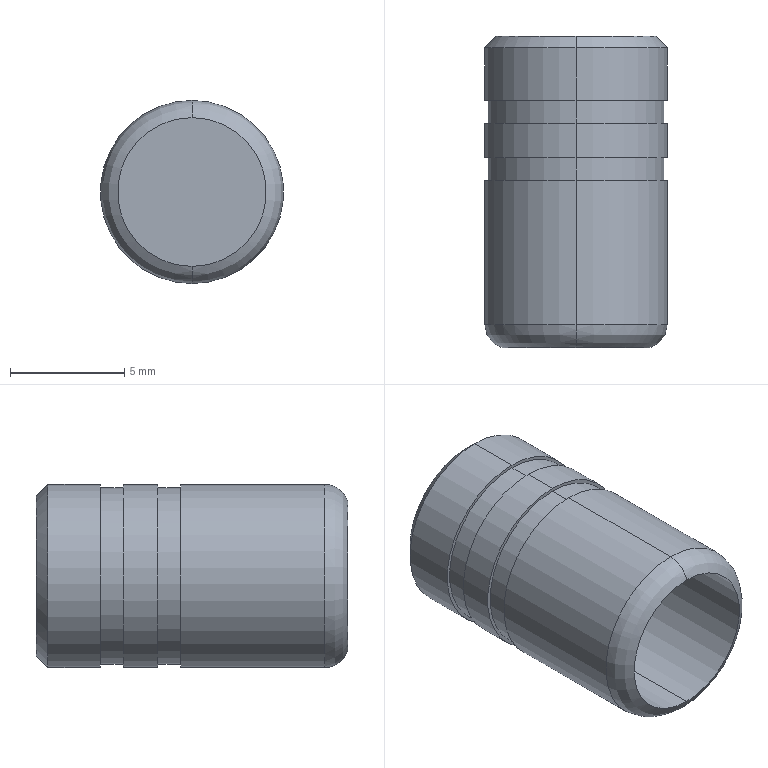Part | SolidWorks | features Revolution 1 | 1 solid | 25 faces | box 8 x 13.6 x 8 mm | volume 252.417 mm3 | cylinder 12 | plane 7 | cone 4 | torus 2 | commonest cylinder face diameters 8 x6 7.7 x4 6.5 x2
STEP:
#1=CARTESIAN_POINT('',(0.,7.3,-4.));
#2=VERTEX_POINT('',#1);
#3=CARTESIAN_POINT('',(0.,7.3,4.));
#4=VERTEX_POINT('',#3);
#5=CARTESIAN_POINT('',(0.,7.3,0.));
#6=DIRECTION('',(0.,-1.,0.));
#7=DIRECTION('',(0.,0.,-1.));
#8=AXIS2_PLACEMENT_3D('',#5,#6,#7);
#9=CIRCLE('',#8,4.);
#10=EDGE_CURVE('',#2,#4,#9,.T.);
#11=ORIENTED_EDGE('',*,*,#10,.T.);
#12=CARTESIAN_POINT('',(0.,1.,4.));
#13=VERTEX_POINT('',#12);
#14=CARTESIAN_POINT('',(0.,0.,4.));
#15=DIRECTION('',(0.,-1.,0.));
#16=VECTOR('',#15,1000.);
#17=LINE('',#14,#16);
#18=EDGE_CURVE('',#4,#13,#17,.T.);
#19=ORIENTED_EDGE('',*,*,#18,.T.);
#20=CARTESIAN_POINT('',(0.,1.,-4.));
#21=VERTEX_POINT('',#20);
#22=CARTESIAN_POINT('',(0.,1.,0.));
#23=DIRECTION('',(0.,-1.,0.));
#24=DIRECTION('',(0.,0.,-1.));
#25=AXIS2_PLACEMENT_3D('',#22,#23,#24);
#26=CIRCLE('',#25,4.);
#27=EDGE_CURVE('',#21,#13,#26,.T.);
#28=ORIENTED_EDGE('',*,*,#27,.F.);
#29=CARTESIAN_POINT('',(0.,0.,-4.));
#30=DIRECTION('',(0.,-1.,0.));
#31=VECTOR('',#30,1000.);
#32=LINE('',#29,#31);
#33=EDGE_CURVE('',#2,#21,#32,.T.);
#34=ORIENTED_EDGE('',*,*,#33,.F.);
#35=EDGE_LOOP('',(#11,#19,#28,#34));
#36=FACE_OUTER_BOUND('',#35,.T.);
#37=CARTESIAN_POINT('',(0.,0.,0.));
#38=DIRECTION('',(0.,-1.,0.));
#39=DIRECTION('',(0.,0.,-1.));
#40=AXIS2_PLACEMENT_3D('',#37,#38,#39);
#41=CYLINDRICAL_SURFACE('',#40,4.);
#42=ADVANCED_FACE('',(#36),#41,.T.);
#43=CARTESIAN_POINT('',(0.,8.3,-3.85));
#44=VERTEX_POINT('',#43);
#45=CARTESIAN_POINT('',(0.,8.3,3.85));
#46=VERTEX_POINT('',#45);
#47=CARTESIAN_POINT('',(0.,8.3,0.));
#48=DIRECTION('',(0.,-1.,0.));
#49=DIRECTION('',(0.,0.,-1.));
#50=AXIS2_PLACEMENT_3D('',#47,#48,#49);
#51=CIRCLE('',#50,3.85);
#52=EDGE_CURVE('',#44,#46,#51,.T.);
#53=ORIENTED_EDGE('',*,*,#52,.T.);
#54=CARTESIAN_POINT('',(0.,7.3,3.85));
#55=VERTEX_POINT('',#54);
#56=CARTESIAN_POINT('',(0.,0.,3.85));
#57=DIRECTION('',(0.,-1.,0.));
#58=VECTOR('',#57,1000.);
#59=LINE('',#56,#58);
#60=EDGE_CURVE('',#46,#55,#59,.T.);
#61=ORIENTED_EDGE('',*,*,#60,.T.);
#62=CARTESIAN_POINT('',(0.,7.3,-3.85));
#63=VERTEX_POINT('',#62);
#64=CARTESIAN_POINT('',(0.,7.3,0.));
#65=DIRECTION('',(0.,-1.,0.));
#66=DIRECTION('',(0.,0.,-1.));
#67=AXIS2_PLACEMENT_3D('',#64,#65,#66);
#68=CIRCLE('',#67,3.85);
#69=EDGE_CURVE('',#63,#55,#68,.T.);
#70=ORIENTED_EDGE('',*,*,#69,.F.);
#71=CARTESIAN_POINT('',(0.,0.,-3.85));
#72=DIRECTION('',(0.,-1.,0.));
#73=VECTOR('',#72,1000.);
#74=LINE('',#71,#73);
#75=EDGE_CURVE('',#44,#63,#74,.T.);
#76=ORIENTED_EDGE('',*,*,#75,.F.);
#77=EDGE_LOOP('',(#53,#61,#70,#76));
#78=FACE_OUTER_BOUND('',#77,.T.);
#79=CARTESIAN_POINT('',(0.,0.,0.));
#80=DIRECTION('',(0.,-1.,0.));
#81=DIRECTION('',(0.,0.,-1.));
#82=AXIS2_PLACEMENT_3D('',#79,#80,#81);
#83=CYLINDRICAL_SURFACE('',#82,3.85);
#84=ADVANCED_FACE('',(#78),#83,.T.);
#85=CARTESIAN_POINT('',(0.,9.8,-4.));
#86=VERTEX_POINT('',#85);
#87=CARTESIAN_POINT('',(0.,9.8,4.));
#88=VERTEX_POINT('',#87);
#89=CARTESIAN_POINT('',(0.,9.8,0.));
#90=DIRECTION('',(0.,-1.,0.));
#91=DIRECTION('',(0.,0.,-1.));
#92=AXIS2_PLACEMENT_3D('',#89,#90,#91);
#93=CIRCLE('',#92,4.);
#94=EDGE_CURVE('',#86,#88,#93,.T.);
#95=ORIENTED_EDGE('',*,*,#94,.T.);
#96=CARTESIAN_POINT('',(0.,8.3,4.));
#97=VERTEX_POINT('',#96);
#98=CARTESIAN_POINT('',(0.,0.,4.));
#99=DIRECTION('',(0.,-1.,0.));
#100=VECTOR('',#99,1000.);
#101=LINE('',#98,#100);
#102=EDGE_CURVE('',#88,#97,#101,.T.);
#103=ORIENTED_EDGE('',*,*,#102,.T.);
#104=CARTESIAN_POINT('',(0.,8.3,-4.));
#105=VERTEX_POINT('',#104);
#106=CARTESIAN_POINT('',(0.,8.3,0.));
#107=DIRECTION('',(0.,-1.,0.));
#108=DIRECTION('',(0.,0.,-1.));
#109=AXIS2_PLACEMENT_3D('',#106,#107,#108);
#110=CIRCLE('',#109,4.);
#111=EDGE_CURVE('',#105,#97,#110,.T.);
#112=ORIENTED_EDGE('',*,*,#111,.F.);
#113=CARTESIAN_POINT('',(0.,0.,-4.));
#114=DIRECTION('',(0.,-1.,0.));
#115=VECTOR('',#114,1000.);
#116=LINE('',#113,#115);
#117=EDGE_CURVE('',#86,#105,#116,.T.);
#118=ORIENTED_EDGE('',*,*,#117,.F.);
#119=EDGE_LOOP('',(#95,#103,#112,#118));
#120=FACE_OUTER_BOUND('',#119,.T.);
#121=CARTESIAN_POINT('',(0.,0.,0.));
#122=DIRECTION('',(0.,-1.,0.));
#123=DIRECTION('',(0.,0.,-1.));
#124=AXIS2_PLACEMENT_3D('',#121,#122,#123);
#125=CYLINDRICAL_SURFACE('',#124,4.);
#126=ADVANCED_FACE('',(#120),#125,.T.);
#127=CARTESIAN_POINT('',(0.,10.8,-3.85));
#128=VERTEX_POINT('',#127);
#129=CARTESIAN_POINT('',(0.,10.8,3.85));
#130=VERTEX_POINT('',#129);
#131=CARTESIAN_POINT('',(0.,10.8,0.));
#132=DIRECTION('',(0.,-1.,0.));
#133=DIRECTION('',(0.,0.,-1.));
#134=AXIS2_PLACEMENT_3D('',#131,#132,#133);
#135=CIRCLE('',#134,3.85);
#136=EDGE_CURVE('',#128,#130,#135,.T.);
#137=ORIENTED_EDGE('',*,*,#136,.T.);
#138=CARTESIAN_POINT('',(0.,9.8,3.85));
#139=VERTEX_POINT('',#138);
#140=CARTESIAN_POINT('',(0.,0.,3.85));
#141=DIRECTION('',(0.,-1.,0.));
#142=VECTOR('',#141,1000.);
#143=LINE('',#140,#142);
#144=EDGE_CURVE('',#130,#139,#143,.T.);
#145=ORIENTED_EDGE('',*,*,#144,.T.);
#146=CARTESIAN_POINT('',(0.,9.8,-3.85));
#147=VERTEX_POINT('',#146);
#148=CARTESIAN_POINT('',(0.,9.8,0.));
#149=DIRECTION('',(0.,-1.,0.));
#150=DIRECTION('',(0.,0.,-1.));
#151=AXIS2_PLACEMENT_3D('',#148,#149,#150);
#152=CIRCLE('',#151,3.85);
#153=EDGE_CURVE('',#147,#139,#152,.T.);
#154=ORIENTED_EDGE('',*,*,#153,.F.);
#155=CARTESIAN_POINT('',(0.,0.,-3.85));
#156=DIRECTION('',(0.,-1.,0.));
#157=VECTOR('',#156,1000.);
#158=LINE('',#155,#157);
#159=EDGE_CURVE('',#128,#147,#158,.T.);
#160=ORIENTED_EDGE('',*,*,#159,.F.);
#161=EDGE_LOOP('',(#137,#145,#154,#160));
#162=FACE_OUTER_BOUND('',#161,.T.);
#163=CARTESIAN_POINT('',(0.,0.,0.));
#164=DIRECTION('',(0.,-1.,0.));
#165=DIRECTION('',(0.,0.,-1.));
#166=AXIS2_PLACEMENT_3D('',#163,#164,#165);
#167=CYLINDRICAL_SURFACE('',#166,3.85);
#168=ADVANCED_FACE('',(#162),#167,.T.);
#169=CARTESIAN_POINT('',(0.,13.1,-4.));
#170=VERTEX_POINT('',#169);
#171=CARTESIAN_POINT('',(0.,13.1,4.));
#172=VERTEX_POINT('',#171);
#173=CARTESIAN_POINT('',(0.,13.1,0.));
#174=DIRECTION('',(0.,-1.,0.));
#175=DIRECTION('',(0.,0.,-1.));
#176=AXIS2_PLACEMENT_3D('',#173,#174,#175);
#177=CIRCLE('',#176,4.);
#178=EDGE_CURVE('',#170,#172,#177,.T.);
#179=ORIENTED_EDGE('',*,*,#178,.T.);
#180=CARTESIAN_POINT('',(0.,10.8,4.));
#181=VERTEX_POINT('',#180);
#182=CARTESIAN_POINT('',(0.,0.,4.));
#183=DIRECTION('',(0.,-1.,0.));
#184=VECTOR('',#183,1000.);
#185=LINE('',#182,#184);
#186=EDGE_CURVE('',#172,#181,#185,.T.);
#187=ORIENTED_EDGE('',*,*,#186,.T.);
#188=CARTESIAN_POINT('',(0.,10.8,-4.));
#189=VERTEX_POINT('',#188);
#190=CARTESIAN_POINT('',(0.,10.8,0.));
#191=DIRECTION('',(0.,-1.,0.));
#192=DIRECTION('',(0.,0.,-1.));
#193=AXIS2_PLACEMENT_3D('',#190,#191,#192);
#194=CIRCLE('',#193,4.);
#195=EDGE_CURVE('',#189,#181,#194,.T.);
#196=ORIENTED_EDGE('',*,*,#195,.F.);
#197=CARTESIAN_POINT('',(0.,0.,-4.));
#198=DIRECTION('',(0.,-1.,0.));
#199=VECTOR('',#198,1000.);
#200=LINE('',#197,#199);
#201=EDGE_CURVE('',#170,#189,#200,.T.);
#202=ORIENTED_EDGE('',*,*,#201,.F.);
#203=EDGE_LOOP('',(#179,#187,#196,#202));
#204=FACE_OUTER_BOUND('',#203,.T.);
#205=CARTESIAN_POINT('',(0.,0.,0.));
#206=DIRECTION('',(0.,-1.,0.));
#207=DIRECTION('',(0.,0.,-1.));
#208=AXIS2_PLACEMENT_3D('',#205,#206,#207);
#209=CYLINDRICAL_SURFACE('',#208,4.);
#210=ADVANCED_FACE('',(#204),#209,.T.);
#211=CARTESIAN_POINT('',(0.,13.6,-3.5));
#212=VERTEX_POINT('',#211);
#213=CARTESIAN_POINT('',(0.,13.6,3.5));
#214=VERTEX_POINT('',#213);
#215=CARTESIAN_POINT('',(0.,13.6,0.));
#216=DIRECTION('',(0.,-1.,0.));
#217=DIRECTION('',(0.,0.,-1.));
#218=AXIS2_PLACEMENT_3D('',#215,#216,#217);
#219=CIRCLE('',#218,3.5);
#220=EDGE_CURVE('',#212,#214,#219,.T.);
#221=ORIENTED_EDGE('',*,*,#220,.T.);
#222=CARTESIAN_POINT('',(0.,13.6,3.5));
#223=DIRECTION('',(0.,-0.7071,0.7071));
#224=VECTOR('',#223,1000.);
#225=LINE('',#222,#224);
#226=EDGE_CURVE('',#214,#172,#225,.T.);
#227=ORIENTED_EDGE('',*,*,#226,.T.);
#228=ORIENTED_EDGE('',*,*,#178,.F.);
#229=CARTESIAN_POINT('',(0.,13.6,-3.5));
#230=DIRECTION('',(0.,-0.7071,-0.7071));
#231=VECTOR('',#230,1000.);
#232=LINE('',#229,#231);
#233=EDGE_CURVE('',#212,#170,#232,.T.);
#234=ORIENTED_EDGE('',*,*,#233,.F.);
#235=EDGE_LOOP('',(#221,#227,#228,#234));
#236=FACE_OUTER_BOUND('',#235,.T.);
#237=CARTESIAN_POINT('',(0.,13.6,0.));
#238=DIRECTION('',(0.,-1.,0.));
#239=DIRECTION('',(0.,0.,-1.));
#240=AXIS2_PLACEMENT_3D('',#237,#238,#239);
#241=CONICAL_SURFACE('',#240,3.5,0.7854);
#242=ADVANCED_FACE('',(#236),#241,.T.);
#243=CARTESIAN_POINT('',(0.,13.1,0.5));
#244=VERTEX_POINT('',#243);
#245=CARTESIAN_POINT('',(0.,13.1,-0.5));
#246=VERTEX_POINT('',#245);
#247=CARTESIAN_POINT('',(0.,13.1,0.));
#248=DIRECTION('',(0.,-1.,0.));
#249=DIRECTION('',(0.,0.,-1.));
#250=AXIS2_PLACEMENT_3D('',#247,#248,#249);
#251=CIRCLE('',#250,0.5);
#252=EDGE_CURVE('',#244,#246,#251,.T.);
#253=ORIENTED_EDGE('',*,*,#252,.T.);
#254=CARTESIAN_POINT('',(0.,13.6,-1.25));
#255=VERTEX_POINT('',#254);
#256=CARTESIAN_POINT('',(0.,13.1,-0.5));
#257=DIRECTION('',(0.,0.5547,-0.8321));
#258=VECTOR('',#257,1000.);
#259=LINE('',#256,#258);
#260=EDGE_CURVE('',#246,#255,#259,.T.);
#261=ORIENTED_EDGE('',*,*,#260,.T.);
#262=CARTESIAN_POINT('',(0.,13.6,1.25));
#263=VERTEX_POINT('',#262);
#264=CARTESIAN_POINT('',(0.,13.6,0.));
#265=DIRECTION('',(0.,-1.,0.));
#266=DIRECTION('',(0.,0.,-1.));
#267=AXIS2_PLACEMENT_3D('',#264,#265,#266);
#268=CIRCLE('',#267,1.25);
#269=EDGE_CURVE('',#263,#255,#268,.T.);
#270=ORIENTED_EDGE('',*,*,#269,.F.);
#271=CARTESIAN_POINT('',(0.,13.1,0.5));
#272=DIRECTION('',(0.,0.5547,0.8321));
#273=VECTOR('',#272,1000.);
#274=LINE('',#271,#273);
#275=EDGE_CURVE('',#244,#263,#274,.T.);
#276=ORIENTED_EDGE('',*,*,#275,.F.);
#277=EDGE_LOOP('',(#253,#261,#270,#276));
#278=FACE_OUTER_BOUND('',#277,.T.);
#279=CARTESIAN_POINT('',(0.,13.1,0.));
#280=DIRECTION('',(0.,1.,0.));
#281=DIRECTION('',(0.,0.,1.));
#282=AXIS2_PLACEMENT_3D('',#279,#280,#281);
#283=CONICAL_SURFACE('',#282,0.5,0.9828);
#284=ADVANCED_FACE('',(#278),#283,.F.);
#285=CARTESIAN_POINT('',(0.,12.5,3.25));
#286=VERTEX_POINT('',#285);
#287=CARTESIAN_POINT('',(0.,12.5,-3.25));
#288=VERTEX_POINT('',#287);
#289=CARTESIAN_POINT('',(0.,12.5,0.));
#290=DIRECTION('',(0.,-1.,0.));
#291=DIRECTION('',(0.,0.,-1.));
#292=AXIS2_PLACEMENT_3D('',#289,#290,#291);
#293=CIRCLE('',#292,3.25);
#294=EDGE_CURVE('',#286,#288,#293,.T.);
#295=ORIENTED_EDGE('',*,*,#294,.F.);
#296=CARTESIAN_POINT('',(0.,0.,3.25));
#297=VERTEX_POINT('',#296);
#298=CARTESIAN_POINT('',(0.,0.,3.25));
#299=DIRECTION('',(0.,-1.,0.));
#300=VECTOR('',#299,1000.);
#301=LINE('',#298,#300);
#302=EDGE_CURVE('',#286,#297,#301,.T.);
#303=ORIENTED_EDGE('',*,*,#302,.T.);
#304=CARTESIAN_POINT('',(0.,0.,-3.25));
#305=VERTEX_POINT('',#304);
#306=CARTESIAN_POINT('',(0.,0.,0.));
#307=DIRECTION('',(0.,-1.,0.));
#308=DIRECTION('',(0.,0.,-1.));
#309=AXIS2_PLACEMENT_3D('',#306,#307,#308);
#310=CIRCLE('',#309,3.25);
#311=EDGE_CURVE('',#297,#305,#310,.T.);
#312=ORIENTED_EDGE('',*,*,#311,.T.);
#313=CARTESIAN_POINT('',(0.,0.,-3.25));
#314=DIRECTION('',(0.,-1.,0.));
#315=VECTOR('',#314,1000.);
#316=LINE('',#313,#315);
#317=EDGE_CURVE('',#288,#305,#316,.T.);
#318=ORIENTED_EDGE('',*,*,#317,.F.);
#319=EDGE_LOOP('',(#295,#303,#312,#318));
#320=FACE_OUTER_BOUND('',#319,.T.);
#321=CARTESIAN_POINT('',(0.,0.,0.));
#322=DIRECTION('',(0.,-1.,0.));
#323=DIRECTION('',(0.,0.,-1.));
#324=AXIS2_PLACEMENT_3D('',#321,#322,#323);
#325=CYLINDRICAL_SURFACE('',#324,3.25);
#326=ADVANCED_FACE('',(#320),#325,.F.);
#327=ORIENTED_EDGE('',*,*,#27,.T.);
#328=CARTESIAN_POINT('',(0.,1.,2.958));
#329=DIRECTION('',(1.,0.,0.));
#330=DIRECTION('',(0.,0.,-1.));
#331=AXIS2_PLACEMENT_3D('',#328,#329,#330);
#332=CIRCLE('',#331,1.042);
#333=EDGE_CURVE('',#13,#297,#332,.T.);
#334=ORIENTED_EDGE('',*,*,#333,.T.);
#335=CARTESIAN_POINT('',(0.,0.,0.));
#336=DIRECTION('',(0.,-1.,0.));
#337=DIRECTION('',(0.,0.,-1.));
#338=AXIS2_PLACEMENT_3D('',#335,#336,#337);
#339=CIRCLE('',#338,3.25);
#340=EDGE_CURVE('',#305,#297,#339,.T.);
#341=ORIENTED_EDGE('',*,*,#340,.F.);
#342=CARTESIAN_POINT('',(0.,1.,-2.958));
#343=DIRECTION('',(-1.,0.,0.));
#344=DIRECTION('',(0.,0.,1.));
#345=AXIS2_PLACEMENT_3D('',#342,#343,#344);
#346=CIRCLE('',#345,1.042);
#347=EDGE_CURVE('',#21,#305,#346,.T.);
#348=ORIENTED_EDGE('',*,*,#347,.F.);
#349=EDGE_LOOP('',(#327,#334,#341,#348));
#350=FACE_OUTER_BOUND('',#349,.T.);
#351=CARTESIAN_POINT('',(0.,1.,0.));
#352=DIRECTION('',(0.,-1.,0.));
#353=DIRECTION('',(0.,0.,-1.));
#354=AXIS2_PLACEMENT_3D('',#351,#352,#353);
#355=TOROIDAL_SURFACE('',#354,2.958,1.042);
#356=ADVANCED_FACE('',(#350),#355,.T.);
#357=ORIENTED_EDGE('',*,*,#333,.F.);
#358=CARTESIAN_POINT('',(0.,1.,0.));
#359=DIRECTION('',(0.,-1.,0.));
#360=DIRECTION('',(0.,0.,-1.));
#361=AXIS2_PLACEMENT_3D('',#358,#359,#360);
#362=CIRCLE('',#361,4.);
#363=EDGE_CURVE('',#13,#21,#362,.T.);
#364=ORIENTED_EDGE('',*,*,#363,.T.);
#365=ORIENTED_EDGE('',*,*,#347,.T.);
#366=ORIENTED_EDGE('',*,*,#311,.F.);
#367=EDGE_LOOP('',(#357,#364,#365,#366));
#368=FACE_OUTER_BOUND('',#367,.T.);
#369=CARTESIAN_POINT('',(0.,1.,0.));
#370=DIRECTION('',(0.,-1.,0.));
#371=DIRECTION('',(0.,0.,-1.));
#372=AXIS2_PLACEMENT_3D('',#369,#370,#371);
#373=TOROIDAL_SURFACE('',#372,2.958,1.042);
#374=ADVANCED_FACE('',(#368),#373,.T.);
#375=ORIENTED_EDGE('',*,*,#302,.F.);
#376=CARTESIAN_POINT('',(0.,12.5,0.));
#377=DIRECTION('',(0.,-1.,0.));
#378=DIRECTION('',(0.,0.,-1.));
#379=AXIS2_PLACEMENT_3D('',#376,#377,#378);
#380=CIRCLE('',#379,3.25);
#381=EDGE_CURVE('',#288,#286,#380,.T.);
#382=ORIENTED_EDGE('',*,*,#381,.F.);
#383=ORIENTED_EDGE('',*,*,#317,.T.);
#384=ORIENTED_EDGE('',*,*,#340,.T.);
#385=EDGE_LOOP('',(#375,#382,#383,#384));
#386=FACE_OUTER_BOUND('',#385,.T.);
#387=CARTESIAN_POINT('',(0.,0.,0.));
#388=DIRECTION('',(0.,-1.,0.));
#389=DIRECTION('',(0.,0.,-1.));
#390=AXIS2_PLACEMENT_3D('',#387,#388,#389);
#391=CYLINDRICAL_SURFACE('',#390,3.25);
#392=ADVANCED_FACE('',(#386),#391,.F.);
#393=ORIENTED_EDGE('',*,*,#381,.T.);
#394=ORIENTED_EDGE('',*,*,#294,.T.);
#395=EDGE_LOOP('',(#393,#394));
#396=FACE_OUTER_BOUND('',#395,.T.);
#397=CARTESIAN_POINT('',(-3.25,12.5,0.));
#398=DIRECTION('',(0.,1.,0.));
#399=DIRECTION('',(0.,0.,1.));
#400=AXIS2_PLACEMENT_3D('',#397,#398,#399);
#401=PLANE('',#400);
#402=ADVANCED_FACE('',(#396),#401,.F.);
#403=ORIENTED_EDGE('',*,*,#252,.F.);
#404=CARTESIAN_POINT('',(0.,13.1,0.));
#405=DIRECTION('',(0.,-1.,0.));
#406=DIRECTION('',(0.,0.,-1.));
#407=AXIS2_PLACEMENT_3D('',#404,#405,#406);
#408=CIRCLE('',#407,0.5);
#409=EDGE_CURVE('',#246,#244,#408,.T.);
#410=ORIENTED_EDGE('',*,*,#409,.F.);
#411=EDGE_LOOP('',(#403,#410));
#412=FACE_OUTER_BOUND('',#411,.T.);
#413=CARTESIAN_POINT('',(-0.5,13.1,0.));
#414=DIRECTION('',(0.,-1.,0.));
#415=DIRECTION('',(0.,0.,-1.));
#416=AXIS2_PLACEMENT_3D('',#413,#414,#415);
#417=PLANE('',#416);
#418=ADVANCED_FACE('',(#412),#417,.F.);
#419=ORIENTED_EDGE('',*,*,#260,.F.);
#420=ORIENTED_EDGE('',*,*,#409,.T.);
#421=ORIENTED_EDGE('',*,*,#275,.T.);
#422=CARTESIAN_POINT('',(0.,13.6,0.));
#423=DIRECTION('',(0.,-1.,0.));
#424=DIRECTION('',(0.,0.,-1.));
#425=AXIS2_PLACEMENT_3D('',#422,#423,#424);
#426=CIRCLE('',#425,1.25);
#427=EDGE_CURVE('',#255,#263,#426,.T.);
#428=ORIENTED_EDGE('',*,*,#427,.F.);
#429=EDGE_LOOP('',(#419,#420,#421,#428));
#430=FACE_OUTER_BOUND('',#429,.T.);
#431=CARTESIAN_POINT('',(0.,13.1,0.));
#432=DIRECTION('',(0.,1.,0.));
#433=DIRECTION('',(0.,0.,1.));
#434=AXIS2_PLACEMENT_3D('',#431,#432,#433);
#435=CONICAL_SURFACE('',#434,0.5,0.9828);
#436=ADVANCED_FACE('',(#430),#435,.F.);
#437=ORIENTED_EDGE('',*,*,#220,.F.);
#438=CARTESIAN_POINT('',(0.,13.6,0.));
#439=DIRECTION('',(0.,-1.,0.));
#440=DIRECTION('',(0.,0.,-1.));
#441=AXIS2_PLACEMENT_3D('',#438,#439,#440);
#442=CIRCLE('',#441,3.5);
#443=EDGE_CURVE('',#214,#212,#442,.T.);
#444=ORIENTED_EDGE('',*,*,#443,.F.);
#445=EDGE_LOOP('',(#437,#444));
#446=FACE_OUTER_BOUND('',#445,.T.);
#447=ORIENTED_EDGE('',*,*,#269,.T.);
#448=ORIENTED_EDGE('',*,*,#427,.T.);
#449=EDGE_LOOP('',(#447,#448));
#450=FACE_BOUND('',#449,.T.);
#451=CARTESIAN_POINT('',(-3.5,13.6,0.));
#452=DIRECTION('',(0.,-1.,0.));
#453=DIRECTION('',(0.,0.,-1.));
#454=AXIS2_PLACEMENT_3D('',#451,#452,#453);
#455=PLANE('',#454);
#456=ADVANCED_FACE('',(#446,#450),#455,.F.);
#457=ORIENTED_EDGE('',*,*,#226,.F.);
#458=ORIENTED_EDGE('',*,*,#443,.T.);
#459=ORIENTED_EDGE('',*,*,#233,.T.);
#460=CARTESIAN_POINT('',(0.,13.1,0.));
#461=DIRECTION('',(0.,-1.,0.));
#462=DIRECTION('',(0.,0.,-1.));
#463=AXIS2_PLACEMENT_3D('',#460,#461,#462);
#464=CIRCLE('',#463,4.);
#465=EDGE_CURVE('',#172,#170,#464,.T.);
#466=ORIENTED_EDGE('',*,*,#465,.F.);
#467=EDGE_LOOP('',(#457,#458,#459,#466));
#468=FACE_OUTER_BOUND('',#467,.T.);
#469=CARTESIAN_POINT('',(0.,13.6,0.));
#470=DIRECTION('',(0.,-1.,0.));
#471=DIRECTION('',(0.,0.,-1.));
#472=AXIS2_PLACEMENT_3D('',#469,#470,#471);
#473=CONICAL_SURFACE('',#472,3.5,0.7854);
#474=ADVANCED_FACE('',(#468),#473,.T.);
#475=ORIENTED_EDGE('',*,*,#186,.F.);
#476=ORIENTED_EDGE('',*,*,#465,.T.);
#477=ORIENTED_EDGE('',*,*,#201,.T.);
#478=CARTESIAN_POINT('',(0.,10.8,0.));
#479=DIRECTION('',(0.,-1.,0.));
#480=DIRECTION('',(0.,0.,-1.));
#481=AXIS2_PLACEMENT_3D('',#478,#479,#480);
#482=CIRCLE('',#481,4.);
#483=EDGE_CURVE('',#181,#189,#482,.T.);
#484=ORIENTED_EDGE('',*,*,#483,.F.);
#485=EDGE_LOOP('',(#475,#476,#477,#484));
#486=FACE_OUTER_BOUND('',#485,.T.);
#487=CARTESIAN_POINT('',(0.,0.,0.));
#488=DIRECTION('',(0.,-1.,0.));
#489=DIRECTION('',(0.,0.,-1.));
#490=AXIS2_PLACEMENT_3D('',#487,#488,#489);
#491=CYLINDRICAL_SURFACE('',#490,4.);
#492=ADVANCED_FACE('',(#486),#491,.T.);
#493=ORIENTED_EDGE('',*,*,#136,.F.);
#494=CARTESIAN_POINT('',(0.,10.8,0.));
#495=DIRECTION('',(0.,-1.,0.));
#496=DIRECTION('',(0.,0.,-1.));
#497=AXIS2_PLACEMENT_3D('',#494,#495,#496);
#498=CIRCLE('',#497,3.85);
#499=EDGE_CURVE('',#130,#128,#498,.T.);
#500=ORIENTED_EDGE('',*,*,#499,.F.);
#501=EDGE_LOOP('',(#493,#500));
#502=FACE_BOUND('',#501,.T.);
#503=ORIENTED_EDGE('',*,*,#195,.T.);
#504=ORIENTED_EDGE('',*,*,#483,.T.);
#505=EDGE_LOOP('',(#503,#504));
#506=FACE_OUTER_BOUND('',#505,.T.);
#507=CARTESIAN_POINT('',(-3.85,10.8,0.));
#508=DIRECTION('',(0.,1.,0.));
#509=DIRECTION('',(0.,0.,1.));
#510=AXIS2_PLACEMENT_3D('',#507,#508,#509);
#511=PLANE('',#510);
#512=ADVANCED_FACE('',(#502,#506),#511,.F.);
#513=ORIENTED_EDGE('',*,*,#144,.F.);
#514=ORIENTED_EDGE('',*,*,#499,.T.);
#515=ORIENTED_EDGE('',*,*,#159,.T.);
#516=CARTESIAN_POINT('',(0.,9.8,0.));
#517=DIRECTION('',(0.,-1.,0.));
#518=DIRECTION('',(0.,0.,-1.));
#519=AXIS2_PLACEMENT_3D('',#516,#517,#518);
#520=CIRCLE('',#519,3.85);
#521=EDGE_CURVE('',#139,#147,#520,.T.);
#522=ORIENTED_EDGE('',*,*,#521,.F.);
#523=EDGE_LOOP('',(#513,#514,#515,#522));
#524=FACE_OUTER_BOUND('',#523,.T.);
#525=CARTESIAN_POINT('',(0.,0.,0.));
#526=DIRECTION('',(0.,-1.,0.));
#527=DIRECTION('',(0.,0.,-1.));
#528=AXIS2_PLACEMENT_3D('',#525,#526,#527);
#529=CYLINDRICAL_SURFACE('',#528,3.85);
#530=ADVANCED_FACE('',(#524),#529,.T.);
#531=ORIENTED_EDGE('',*,*,#94,.F.);
#532=CARTESIAN_POINT('',(0.,9.8,0.));
#533=DIRECTION('',(0.,-1.,0.));
#534=DIRECTION('',(0.,0.,-1.));
#535=AXIS2_PLACEMENT_3D('',#532,#533,#534);
#536=CIRCLE('',#535,4.);
#537=EDGE_CURVE('',#88,#86,#536,.T.);
#538=ORIENTED_EDGE('',*,*,#537,.F.);
#539=EDGE_LOOP('',(#531,#538));
#540=FACE_OUTER_BOUND('',#539,.T.);
#541=ORIENTED_EDGE('',*,*,#153,.T.);
#542=ORIENTED_EDGE('',*,*,#521,.T.);
#543=EDGE_LOOP('',(#541,#542));
#544=FACE_BOUND('',#543,.T.);
#545=CARTESIAN_POINT('',(-4.,9.8,0.));
#546=DIRECTION('',(0.,-1.,0.));
#547=DIRECTION('',(0.,0.,-1.));
#548=AXIS2_PLACEMENT_3D('',#545,#546,#547);
#549=PLANE('',#548);
#550=ADVANCED_FACE('',(#540,#544),#549,.F.);
#551=ORIENTED_EDGE('',*,*,#102,.F.);
#552=ORIENTED_EDGE('',*,*,#537,.T.);
#553=ORIENTED_EDGE('',*,*,#117,.T.);
#554=CARTESIAN_POINT('',(0.,8.3,0.));
#555=DIRECTION('',(0.,-1.,0.));
#556=DIRECTION('',(0.,0.,-1.));
#557=AXIS2_PLACEMENT_3D('',#554,#555,#556);
#558=CIRCLE('',#557,4.);
#559=EDGE_CURVE('',#97,#105,#558,.T.);
#560=ORIENTED_EDGE('',*,*,#559,.F.);
#561=EDGE_LOOP('',(#551,#552,#553,#560));
#562=FACE_OUTER_BOUND('',#561,.T.);
#563=CARTESIAN_POINT('',(0.,0.,0.));
#564=DIRECTION('',(0.,-1.,0.));
#565=DIRECTION('',(0.,0.,-1.));
#566=AXIS2_PLACEMENT_3D('',#563,#564,#565);
#567=CYLINDRICAL_SURFACE('',#566,4.);
#568=ADVANCED_FACE('',(#562),#567,.T.);
#569=ORIENTED_EDGE('',*,*,#52,.F.);
#570=CARTESIAN_POINT('',(0.,8.3,0.));
#571=DIRECTION('',(0.,-1.,0.));
#572=DIRECTION('',(0.,0.,-1.));
#573=AXIS2_PLACEMENT_3D('',#570,#571,#572);
#574=CIRCLE('',#573,3.85);
#575=EDGE_CURVE('',#46,#44,#574,.T.);
#576=ORIENTED_EDGE('',*,*,#575,.F.);
#577=EDGE_LOOP('',(#569,#576));
#578=FACE_BOUND('',#577,.T.);
#579=ORIENTED_EDGE('',*,*,#111,.T.);
#580=ORIENTED_EDGE('',*,*,#559,.T.);
#581=EDGE_LOOP('',(#579,#580));
#582=FACE_OUTER_BOUND('',#581,.T.);
#583=CARTESIAN_POINT('',(-3.85,8.3,0.));
#584=DIRECTION('',(0.,1.,0.));
#585=DIRECTION('',(0.,0.,1.));
#586=AXIS2_PLACEMENT_3D('',#583,#584,#585);
#587=PLANE('',#586);
#588=ADVANCED_FACE('',(#578,#582),#587,.F.);
#589=ORIENTED_EDGE('',*,*,#60,.F.);
#590=ORIENTED_EDGE('',*,*,#575,.T.);
#591=ORIENTED_EDGE('',*,*,#75,.T.);
#592=CARTESIAN_POINT('',(0.,7.3,0.));
#593=DIRECTION('',(0.,-1.,0.));
#594=DIRECTION('',(0.,0.,-1.));
#595=AXIS2_PLACEMENT_3D('',#592,#593,#594);
#596=CIRCLE('',#595,3.85);
#597=EDGE_CURVE('',#55,#63,#596,.T.);
#598=ORIENTED_EDGE('',*,*,#597,.F.);
#599=EDGE_LOOP('',(#589,#590,#591,#598));
#600=FACE_OUTER_BOUND('',#599,.T.);
#601=CARTESIAN_POINT('',(0.,0.,0.));
#602=DIRECTION('',(0.,-1.,0.));
#603=DIRECTION('',(0.,0.,-1.));
#604=AXIS2_PLACEMENT_3D('',#601,#602,#603);
#605=CYLINDRICAL_SURFACE('',#604,3.85);
#606=ADVANCED_FACE('',(#600),#605,.T.);
#607=ORIENTED_EDGE('',*,*,#10,.F.);
#608=CARTESIAN_POINT('',(0.,7.3,0.));
#609=DIRECTION('',(0.,-1.,0.));
#610=DIRECTION('',(0.,0.,-1.));
#611=AXIS2_PLACEMENT_3D('',#608,#609,#610);
#612=CIRCLE('',#611,4.);
#613=EDGE_CURVE('',#4,#2,#612,.T.);
#614=ORIENTED_EDGE('',*,*,#613,.F.);
#615=EDGE_LOOP('',(#607,#614));
#616=FACE_OUTER_BOUND('',#615,.T.);
#617=ORIENTED_EDGE('',*,*,#69,.T.);
#618=ORIENTED_EDGE('',*,*,#597,.T.);
#619=EDGE_LOOP('',(#617,#618));
#620=FACE_BOUND('',#619,.T.);
#621=CARTESIAN_POINT('',(-3.85,7.3,0.));
#622=DIRECTION('',(0.,-1.,0.));
#623=DIRECTION('',(0.,0.,-1.));
#624=AXIS2_PLACEMENT_3D('',#621,#622,#623);
#625=PLANE('',#624);
#626=ADVANCED_FACE('',(#616,#620),#625,.F.);
#627=ORIENTED_EDGE('',*,*,#18,.F.);
#628=ORIENTED_EDGE('',*,*,#613,.T.);
#629=ORIENTED_EDGE('',*,*,#33,.T.);
#630=ORIENTED_EDGE('',*,*,#363,.F.);
#631=EDGE_LOOP('',(#627,#628,#629,#630));
#632=FACE_OUTER_BOUND('',#631,.T.);
#633=CARTESIAN_POINT('',(0.,0.,0.));
#634=DIRECTION('',(0.,-1.,0.));
#635=DIRECTION('',(0.,0.,-1.));
#636=AXIS2_PLACEMENT_3D('',#633,#634,#635);
#637=CYLINDRICAL_SURFACE('',#636,4.);
#638=ADVANCED_FACE('',(#632),#637,.T.);
#639=CLOSED_SHELL('',(#42,#84,#126,#168,#210,#242,#284,#326,#356,#374,#392,#402,#418,#436,#456,#474,#492,#512,#530,#550,#568,#588,#606,#626,#638));
#640=MANIFOLD_SOLID_BREP('',#639);
#641=CARTESIAN_POINT('',(0.,0.,0.));
#642=DIRECTION('',(0.,0.,1.));
#643=DIRECTION('',(1.,0.,0.));
#644=AXIS2_PLACEMENT_3D('',#641,#642,#643);
#645=(LENGTH_UNIT()NAMED_UNIT(*)SI_UNIT(.MILLI.,.METRE.));
#646=UNCERTAINTY_MEASURE_WITH_UNIT(LENGTH_MEASURE(0.00001),#645,'','');
#647=(NAMED_UNIT(*)PLANE_ANGLE_UNIT()SI_UNIT($,.RADIAN.));
#648=(NAMED_UNIT(*)SI_UNIT($,.STERADIAN.)SOLID_ANGLE_UNIT());
#649=(GEOMETRIC_REPRESENTATION_CONTEXT(3)GLOBAL_UNCERTAINTY_ASSIGNED_CONTEXT((#646))GLOBAL_UNIT_ASSIGNED_CONTEXT((#645,#647,#648))REPRESENTATION_CONTEXT('',''));
#650=ADVANCED_BREP_SHAPE_REPRESENTATION('',(#640,#644),#649);